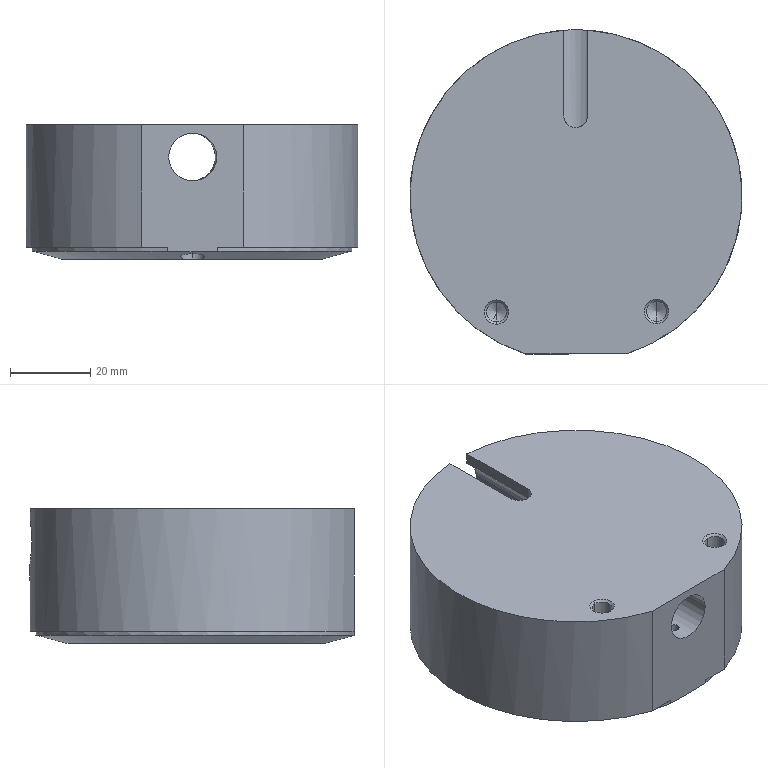Part | SolidWorks | features BaseBody 1 | 1 solid | 50 faces | box 83 x 81.055 x 33.5 mm | volume 151646 mm3 | cylinder 25 | cone 14 | plane 9 | spline 2 | commonest cylinder face diameters 5 x6 6 x5 2.5 x4 3.4 x4 12 x2 20 x2